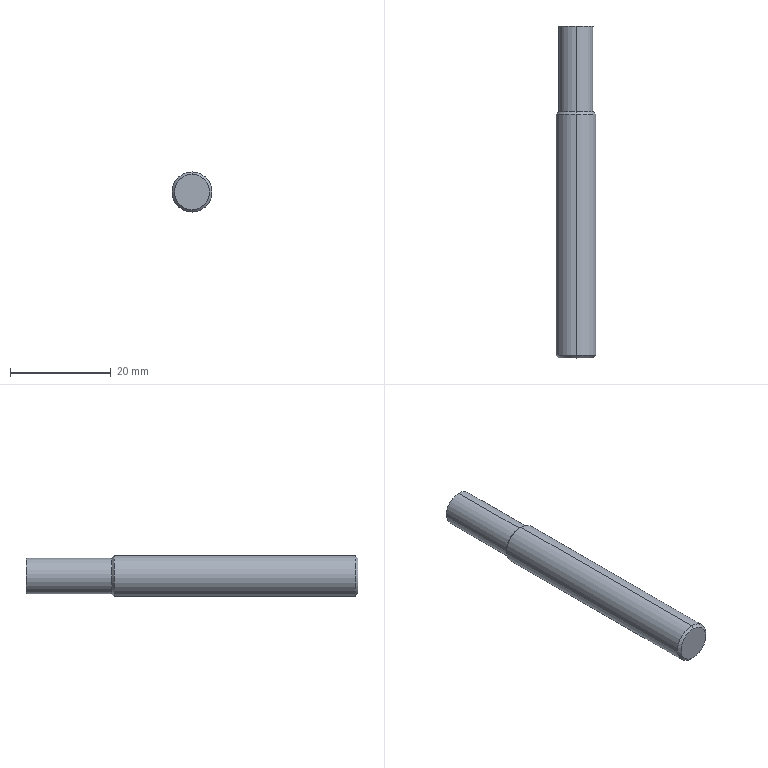Part | SolidWorks | features Chamfer 1, Extrusion 1, ICE 1 | 1 solid | 10 faces | box 8 x 66 x 8 mm | volume 3111 mm3 | cone 4 | cylinder 4 | plane 2 | commonest cylinder face diameters 7 x2 8 x2
STEP:
#1=CARTESIAN_POINT('',(0.,0.,-3.5));
#2=VERTEX_POINT('',#1);
#3=CARTESIAN_POINT('',(0.,0.,3.5));
#4=VERTEX_POINT('',#3);
#5=CARTESIAN_POINT('',(0.,0.,0.));
#6=DIRECTION('',(0.,-1.,0.));
#7=DIRECTION('',(0.,0.,1.));
#8=AXIS2_PLACEMENT_3D('',#5,#6,#7);
#9=CIRCLE('',#8,3.5);
#10=EDGE_CURVE('',#2,#4,#9,.T.);
#11=ORIENTED_EDGE('',*,*,#10,.F.);
#12=CARTESIAN_POINT('',(0.,0.5,-4.));
#13=VERTEX_POINT('',#12);
#14=CARTESIAN_POINT('',(0.,0.5,-4.));
#15=DIRECTION('',(0.,0.7071,-0.7071));
#16=VECTOR('',#15,1000.);
#17=LINE('',#14,#16);
#18=EDGE_CURVE('',#2,#13,#17,.T.);
#19=ORIENTED_EDGE('',*,*,#18,.T.);
#20=CARTESIAN_POINT('',(0.,0.5,4.));
#21=VERTEX_POINT('',#20);
#22=CARTESIAN_POINT('',(0.,0.5,0.));
#23=DIRECTION('',(0.,1.,0.));
#24=DIRECTION('',(0.,0.,1.));
#25=AXIS2_PLACEMENT_3D('',#22,#23,#24);
#26=CIRCLE('',#25,4.);
#27=EDGE_CURVE('',#21,#13,#26,.T.);
#28=ORIENTED_EDGE('',*,*,#27,.F.);
#29=CARTESIAN_POINT('',(0.,0.5,4.));
#30=DIRECTION('',(0.,0.7071,0.7071));
#31=VECTOR('',#30,1000.);
#32=LINE('',#29,#31);
#33=EDGE_CURVE('',#4,#21,#32,.T.);
#34=ORIENTED_EDGE('',*,*,#33,.F.);
#35=EDGE_LOOP('',(#11,#19,#28,#34));
#36=FACE_OUTER_BOUND('',#35,.T.);
#37=CARTESIAN_POINT('',(0.,0.5,0.));
#38=DIRECTION('',(0.,1.,0.));
#39=DIRECTION('',(0.,0.,1.));
#40=AXIS2_PLACEMENT_3D('',#37,#38,#39);
#41=CONICAL_SURFACE('',#40,4.,0.7854);
#42=ADVANCED_FACE('',(#36),#41,.T.);
#43=CARTESIAN_POINT('',(0.,49.,3.5));
#44=VERTEX_POINT('',#43);
#45=CARTESIAN_POINT('',(0.,49.,-3.5));
#46=VERTEX_POINT('',#45);
#47=CARTESIAN_POINT('',(0.,49.,0.));
#48=DIRECTION('',(0.,1.,0.));
#49=DIRECTION('',(0.,0.,1.));
#50=AXIS2_PLACEMENT_3D('',#47,#48,#49);
#51=CIRCLE('',#50,3.5);
#52=EDGE_CURVE('',#44,#46,#51,.T.);
#53=ORIENTED_EDGE('',*,*,#52,.F.);
#54=CARTESIAN_POINT('',(0.,48.5,4.));
#55=VERTEX_POINT('',#54);
#56=CARTESIAN_POINT('',(0.,49.,3.5));
#57=DIRECTION('',(0.,-0.7071,0.7071));
#58=VECTOR('',#57,1000.);
#59=LINE('',#56,#58);
#60=EDGE_CURVE('',#44,#55,#59,.T.);
#61=ORIENTED_EDGE('',*,*,#60,.T.);
#62=CARTESIAN_POINT('',(0.,48.5,-4.));
#63=VERTEX_POINT('',#62);
#64=CARTESIAN_POINT('',(0.,48.5,0.));
#65=DIRECTION('',(0.,-1.,0.));
#66=DIRECTION('',(0.,0.,1.));
#67=AXIS2_PLACEMENT_3D('',#64,#65,#66);
#68=CIRCLE('',#67,4.);
#69=EDGE_CURVE('',#63,#55,#68,.T.);
#70=ORIENTED_EDGE('',*,*,#69,.F.);
#71=CARTESIAN_POINT('',(0.,49.,-3.5));
#72=DIRECTION('',(0.,-0.7071,-0.7071));
#73=VECTOR('',#72,1000.);
#74=LINE('',#71,#73);
#75=EDGE_CURVE('',#46,#63,#74,.T.);
#76=ORIENTED_EDGE('',*,*,#75,.F.);
#77=EDGE_LOOP('',(#53,#61,#70,#76));
#78=FACE_OUTER_BOUND('',#77,.T.);
#79=CARTESIAN_POINT('',(0.,49.,0.));
#80=DIRECTION('',(0.,-1.,0.));
#81=DIRECTION('',(0.,0.,-1.));
#82=AXIS2_PLACEMENT_3D('',#79,#80,#81);
#83=CONICAL_SURFACE('',#82,3.5,0.7854);
#84=ADVANCED_FACE('',(#78),#83,.T.);
#85=CARTESIAN_POINT('',(0.,66.,3.5));
#86=VERTEX_POINT('',#85);
#87=CARTESIAN_POINT('',(0.,66.,-3.5));
#88=VERTEX_POINT('',#87);
#89=CARTESIAN_POINT('',(0.,66.,0.));
#90=DIRECTION('',(0.,1.,0.));
#91=DIRECTION('',(0.,0.,1.));
#92=AXIS2_PLACEMENT_3D('',#89,#90,#91);
#93=CIRCLE('',#92,3.5);
#94=EDGE_CURVE('',#86,#88,#93,.T.);
#95=ORIENTED_EDGE('',*,*,#94,.F.);
#96=CARTESIAN_POINT('',(0.,66.,3.5));
#97=DIRECTION('',(0.,-1.,0.));
#98=VECTOR('',#97,1000.);
#99=LINE('',#96,#98);
#100=EDGE_CURVE('',#86,#44,#99,.T.);
#101=ORIENTED_EDGE('',*,*,#100,.T.);
#102=ORIENTED_EDGE('',*,*,#52,.T.);
#103=CARTESIAN_POINT('',(0.,66.,-3.5));
#104=DIRECTION('',(0.,-1.,0.));
#105=VECTOR('',#104,1000.);
#106=LINE('',#103,#105);
#107=EDGE_CURVE('',#88,#46,#106,.T.);
#108=ORIENTED_EDGE('',*,*,#107,.F.);
#109=EDGE_LOOP('',(#95,#101,#102,#108));
#110=FACE_OUTER_BOUND('',#109,.T.);
#111=CARTESIAN_POINT('',(0.,66.,0.));
#112=DIRECTION('',(0.,-1.,0.));
#113=DIRECTION('',(0.,0.,-1.));
#114=AXIS2_PLACEMENT_3D('',#111,#112,#113);
#115=CYLINDRICAL_SURFACE('',#114,3.5);
#116=ADVANCED_FACE('',(#110),#115,.T.);
#117=ORIENTED_EDGE('',*,*,#69,.T.);
#118=CARTESIAN_POINT('',(0.,49.,4.));
#119=DIRECTION('',(0.,-1.,0.));
#120=VECTOR('',#119,1000.);
#121=LINE('',#118,#120);
#122=EDGE_CURVE('',#55,#21,#121,.T.);
#123=ORIENTED_EDGE('',*,*,#122,.T.);
#124=ORIENTED_EDGE('',*,*,#27,.T.);
#125=CARTESIAN_POINT('',(0.,49.,-4.));
#126=DIRECTION('',(0.,-1.,0.));
#127=VECTOR('',#126,1000.);
#128=LINE('',#125,#127);
#129=EDGE_CURVE('',#63,#13,#128,.T.);
#130=ORIENTED_EDGE('',*,*,#129,.F.);
#131=EDGE_LOOP('',(#117,#123,#124,#130));
#132=FACE_OUTER_BOUND('',#131,.T.);
#133=CARTESIAN_POINT('',(0.,49.,0.));
#134=DIRECTION('',(0.,-1.,0.));
#135=DIRECTION('',(0.,0.,-1.));
#136=AXIS2_PLACEMENT_3D('',#133,#134,#135);
#137=CYLINDRICAL_SURFACE('',#136,4.);
#138=ADVANCED_FACE('',(#132),#137,.T.);
#139=ORIENTED_EDGE('',*,*,#122,.F.);
#140=CARTESIAN_POINT('',(0.,48.5,0.));
#141=DIRECTION('',(0.,-1.,0.));
#142=DIRECTION('',(0.,0.,1.));
#143=AXIS2_PLACEMENT_3D('',#140,#141,#142);
#144=CIRCLE('',#143,4.);
#145=EDGE_CURVE('',#55,#63,#144,.T.);
#146=ORIENTED_EDGE('',*,*,#145,.T.);
#147=ORIENTED_EDGE('',*,*,#129,.T.);
#148=CARTESIAN_POINT('',(0.,0.5,0.));
#149=DIRECTION('',(0.,1.,0.));
#150=DIRECTION('',(0.,0.,1.));
#151=AXIS2_PLACEMENT_3D('',#148,#149,#150);
#152=CIRCLE('',#151,4.);
#153=EDGE_CURVE('',#13,#21,#152,.T.);
#154=ORIENTED_EDGE('',*,*,#153,.T.);
#155=EDGE_LOOP('',(#139,#146,#147,#154));
#156=FACE_OUTER_BOUND('',#155,.T.);
#157=CARTESIAN_POINT('',(0.,49.,0.));
#158=DIRECTION('',(0.,-1.,0.));
#159=DIRECTION('',(0.,0.,-1.));
#160=AXIS2_PLACEMENT_3D('',#157,#158,#159);
#161=CYLINDRICAL_SURFACE('',#160,4.);
#162=ADVANCED_FACE('',(#156),#161,.T.);
#163=CARTESIAN_POINT('',(0.,0.,0.));
#164=DIRECTION('',(0.,-1.,0.));
#165=DIRECTION('',(0.,0.,1.));
#166=AXIS2_PLACEMENT_3D('',#163,#164,#165);
#167=CIRCLE('',#166,3.5);
#168=EDGE_CURVE('',#4,#2,#167,.T.);
#169=ORIENTED_EDGE('',*,*,#168,.T.);
#170=ORIENTED_EDGE('',*,*,#10,.T.);
#171=EDGE_LOOP('',(#169,#170));
#172=FACE_OUTER_BOUND('',#171,.T.);
#173=CARTESIAN_POINT('',(0.,0.,0.));
#174=DIRECTION('',(0.,1.,0.));
#175=DIRECTION('',(0.,0.,1.));
#176=AXIS2_PLACEMENT_3D('',#173,#174,#175);
#177=PLANE('',#176);
#178=ADVANCED_FACE('',(#172),#177,.F.);
#179=ORIENTED_EDGE('',*,*,#100,.F.);
#180=CARTESIAN_POINT('',(0.,66.,0.));
#181=DIRECTION('',(0.,1.,0.));
#182=DIRECTION('',(0.,0.,1.));
#183=AXIS2_PLACEMENT_3D('',#180,#181,#182);
#184=CIRCLE('',#183,3.5);
#185=EDGE_CURVE('',#88,#86,#184,.T.);
#186=ORIENTED_EDGE('',*,*,#185,.F.);
#187=ORIENTED_EDGE('',*,*,#107,.T.);
#188=CARTESIAN_POINT('',(0.,49.,0.));
#189=DIRECTION('',(0.,1.,0.));
#190=DIRECTION('',(0.,0.,1.));
#191=AXIS2_PLACEMENT_3D('',#188,#189,#190);
#192=CIRCLE('',#191,3.5);
#193=EDGE_CURVE('',#46,#44,#192,.T.);
#194=ORIENTED_EDGE('',*,*,#193,.T.);
#195=EDGE_LOOP('',(#179,#186,#187,#194));
#196=FACE_OUTER_BOUND('',#195,.T.);
#197=CARTESIAN_POINT('',(0.,66.,0.));
#198=DIRECTION('',(0.,-1.,0.));
#199=DIRECTION('',(0.,0.,-1.));
#200=AXIS2_PLACEMENT_3D('',#197,#198,#199);
#201=CYLINDRICAL_SURFACE('',#200,3.5);
#202=ADVANCED_FACE('',(#196),#201,.T.);
#203=ORIENTED_EDGE('',*,*,#185,.T.);
#204=ORIENTED_EDGE('',*,*,#94,.T.);
#205=EDGE_LOOP('',(#203,#204));
#206=FACE_OUTER_BOUND('',#205,.T.);
#207=CARTESIAN_POINT('',(0.,66.,0.));
#208=DIRECTION('',(0.,1.,0.));
#209=DIRECTION('',(0.,0.,1.));
#210=AXIS2_PLACEMENT_3D('',#207,#208,#209);
#211=PLANE('',#210);
#212=ADVANCED_FACE('',(#206),#211,.T.);
#213=ORIENTED_EDGE('',*,*,#60,.F.);
#214=ORIENTED_EDGE('',*,*,#193,.F.);
#215=ORIENTED_EDGE('',*,*,#75,.T.);
#216=ORIENTED_EDGE('',*,*,#145,.F.);
#217=EDGE_LOOP('',(#213,#214,#215,#216));
#218=FACE_OUTER_BOUND('',#217,.T.);
#219=CARTESIAN_POINT('',(0.,49.,0.));
#220=DIRECTION('',(0.,-1.,0.));
#221=DIRECTION('',(0.,0.,-1.));
#222=AXIS2_PLACEMENT_3D('',#219,#220,#221);
#223=CONICAL_SURFACE('',#222,3.5,0.7854);
#224=ADVANCED_FACE('',(#218),#223,.T.);
#225=ORIENTED_EDGE('',*,*,#18,.F.);
#226=ORIENTED_EDGE('',*,*,#168,.F.);
#227=ORIENTED_EDGE('',*,*,#33,.T.);
#228=ORIENTED_EDGE('',*,*,#153,.F.);
#229=EDGE_LOOP('',(#225,#226,#227,#228));
#230=FACE_OUTER_BOUND('',#229,.T.);
#231=CARTESIAN_POINT('',(0.,0.5,0.));
#232=DIRECTION('',(0.,1.,0.));
#233=DIRECTION('',(0.,0.,1.));
#234=AXIS2_PLACEMENT_3D('',#231,#232,#233);
#235=CONICAL_SURFACE('',#234,4.,0.7854);
#236=ADVANCED_FACE('',(#230),#235,.T.);
#237=CLOSED_SHELL('',(#42,#84,#116,#138,#162,#178,#202,#212,#224,#236));
#238=MANIFOLD_SOLID_BREP('',#237);
#239=CARTESIAN_POINT('',(0.,0.,0.));
#240=DIRECTION('',(0.,0.,1.));
#241=DIRECTION('',(1.,0.,0.));
#242=AXIS2_PLACEMENT_3D('',#239,#240,#241);
#243=(LENGTH_UNIT()NAMED_UNIT(*)SI_UNIT(.MILLI.,.METRE.));
#244=UNCERTAINTY_MEASURE_WITH_UNIT(LENGTH_MEASURE(0.00001),#243,'','');
#245=(NAMED_UNIT(*)PLANE_ANGLE_UNIT()SI_UNIT($,.RADIAN.));
#246=(NAMED_UNIT(*)SI_UNIT($,.STERADIAN.)SOLID_ANGLE_UNIT());
#247=(GEOMETRIC_REPRESENTATION_CONTEXT(3)GLOBAL_UNCERTAINTY_ASSIGNED_CONTEXT((#244))GLOBAL_UNIT_ASSIGNED_CONTEXT((#243,#245,#246))REPRESENTATION_CONTEXT('',''));
#248=ADVANCED_BREP_SHAPE_REPRESENTATION('',(#238,#242),#247);